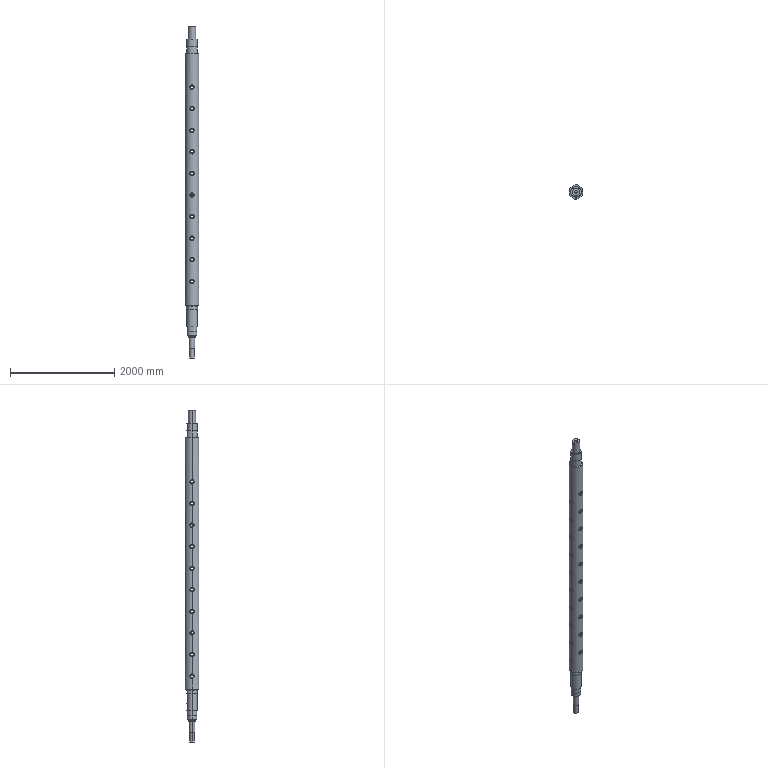Part | SolidWorks | features ICE 15, LPattern 6, MirrorPattern 5, Fillet 2, HoleWzd 2, MoveFace 2, RefAxis 2, Chamfer 1, CombineBodies 1, Extrusion 1, MoveCopyBody 1, Revolution 1, Split 1, WeldBeadFeat 1, WeldmentFeature 1 | 7 solids | 269 faces | box 265 x 265 x 6370 mm | volume 136126152 mm3 | cylinder 194 | plane 63 | cone 8 | torus 4 | commonest cylinder face diameters 50 x82 85 x80 180 x4 200 x4 212 x4 6.8 x2